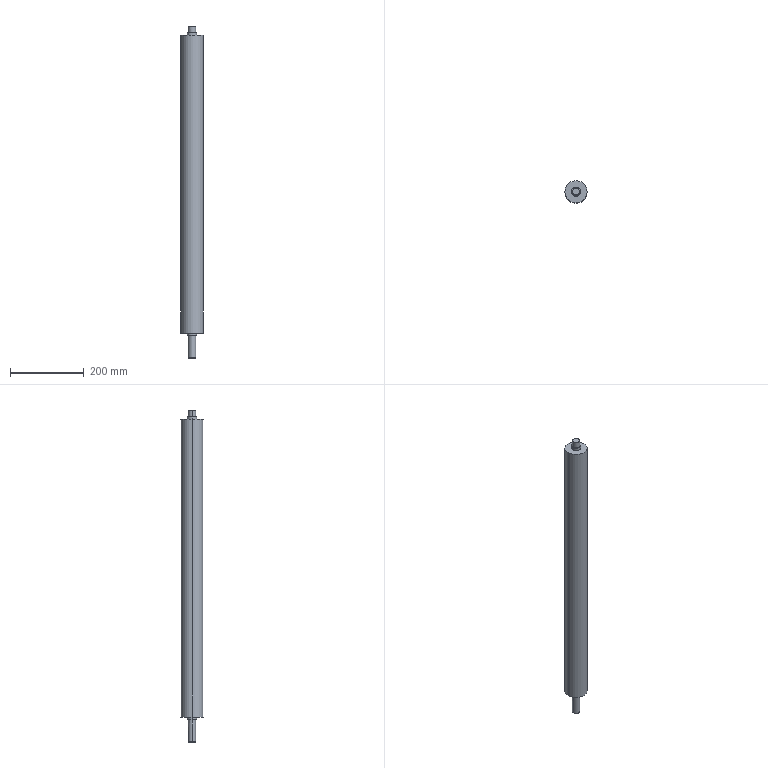Part | STEP file | Main roller | 1 solid | 32 faces | box 60 x 60 x 898 mm | volume 2307157 mm3 | cylinder 14 | cone 9 | plane 9 | commonest cylinder face diameters 20 x4 25 x4 4.134 x2 6 x2 60 x2